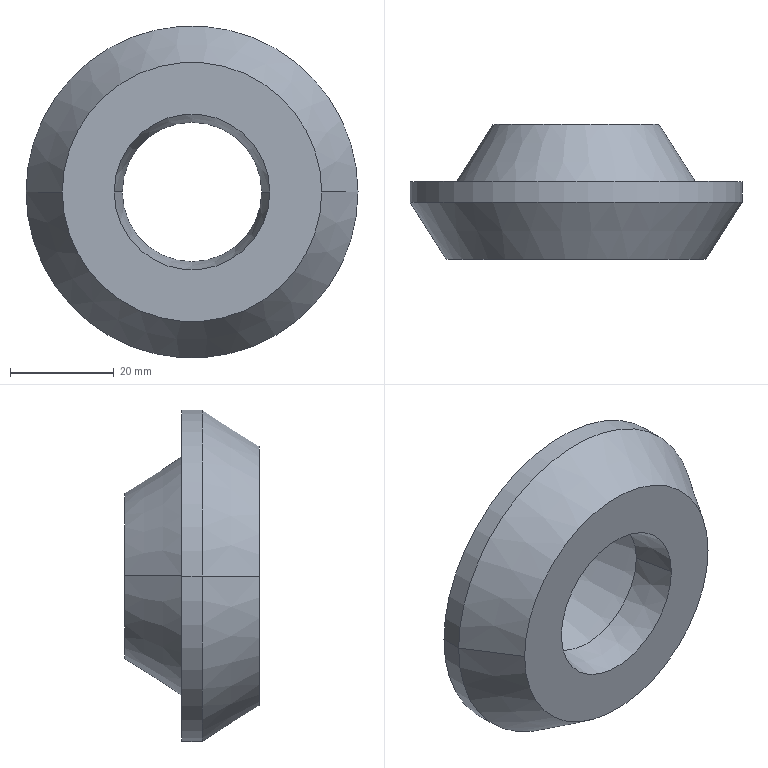Part | SolidWorks | features Revolution 1 | 1 solid | 19 faces | box 64 x 26 x 64 mm | volume 21380 mm3 | cone 12 | plane 5 | cylinder 2 | commonest cylinder face diameters 64 x2
STEP:
#1=CARTESIAN_POINT('',(22.804,4.,0.));
#2=VERTEX_POINT('',#1);
#3=CARTESIAN_POINT('',(-22.804,4.,0.));
#4=VERTEX_POINT('',#3);
#5=CARTESIAN_POINT('',(0.,4.,0.));
#6=DIRECTION('',(0.,1.,0.));
#7=DIRECTION('',(-1.,0.,0.));
#8=AXIS2_PLACEMENT_3D('',#5,#6,#7);
#9=CIRCLE('',#8,22.804);
#10=EDGE_CURVE('',#2,#4,#9,.T.);
#11=ORIENTED_EDGE('',*,*,#10,.F.);
#12=CARTESIAN_POINT('',(27.259,11.,0.));
#13=VERTEX_POINT('',#12);
#14=CARTESIAN_POINT('',(27.259,11.,0.));
#15=DIRECTION('',(0.5369,0.8437,0.));
#16=VECTOR('',#15,1000.);
#17=LINE('',#14,#16);
#18=EDGE_CURVE('',#2,#13,#17,.T.);
#19=ORIENTED_EDGE('',*,*,#18,.T.);
#20=CARTESIAN_POINT('',(-27.259,11.,0.));
#21=VERTEX_POINT('',#20);
#22=CARTESIAN_POINT('',(0.,11.,0.));
#23=DIRECTION('',(0.,1.,0.));
#24=DIRECTION('',(-1.,0.,0.));
#25=AXIS2_PLACEMENT_3D('',#22,#23,#24);
#26=CIRCLE('',#25,27.259);
#27=EDGE_CURVE('',#13,#21,#26,.T.);
#28=ORIENTED_EDGE('',*,*,#27,.T.);
#29=CARTESIAN_POINT('',(-27.259,11.,0.));
#30=DIRECTION('',(-0.5369,0.8437,0.));
#31=VECTOR('',#30,1000.);
#32=LINE('',#29,#31);
#33=EDGE_CURVE('',#4,#21,#32,.T.);
#34=ORIENTED_EDGE('',*,*,#33,.F.);
#35=EDGE_LOOP('',(#11,#19,#28,#34));
#36=FACE_OUTER_BOUND('',#35,.T.);
#37=CARTESIAN_POINT('',(0.,11.,0.));
#38=DIRECTION('',(0.,1.,0.));
#39=DIRECTION('',(-1.,0.,0.));
#40=AXIS2_PLACEMENT_3D('',#37,#38,#39);
#41=CONICAL_SURFACE('',#40,27.259,0.5667);
#42=ADVANCED_FACE('',(#36),#41,.F.);
#43=CARTESIAN_POINT('',(-17.524,8.,0.));
#44=VERTEX_POINT('',#43);
#45=CARTESIAN_POINT('',(17.524,8.,0.));
#46=VERTEX_POINT('',#45);
#47=CARTESIAN_POINT('',(0.,8.,0.));
#48=DIRECTION('',(0.,1.,0.));
#49=DIRECTION('',(-1.,0.,0.));
#50=AXIS2_PLACEMENT_3D('',#47,#48,#49);
#51=CIRCLE('',#50,17.524);
#52=EDGE_CURVE('',#44,#46,#51,.T.);
#53=ORIENTED_EDGE('',*,*,#52,.F.);
#54=CARTESIAN_POINT('',(-18.299,4.,0.));
#55=VERTEX_POINT('',#54);
#56=CARTESIAN_POINT('',(-18.299,4.,0.));
#57=DIRECTION('',(-0.1902,-0.9817,0.));
#58=VECTOR('',#57,1000.);
#59=LINE('',#56,#58);
#60=EDGE_CURVE('',#44,#55,#59,.T.);
#61=ORIENTED_EDGE('',*,*,#60,.T.);
#62=CARTESIAN_POINT('',(18.299,4.,0.));
#63=VERTEX_POINT('',#62);
#64=CARTESIAN_POINT('',(0.,4.,0.));
#65=DIRECTION('',(0.,1.,0.));
#66=DIRECTION('',(-1.,0.,0.));
#67=AXIS2_PLACEMENT_3D('',#64,#65,#66);
#68=CIRCLE('',#67,18.299);
#69=EDGE_CURVE('',#55,#63,#68,.T.);
#70=ORIENTED_EDGE('',*,*,#69,.T.);
#71=CARTESIAN_POINT('',(18.299,4.,0.));
#72=DIRECTION('',(0.1902,-0.9817,0.));
#73=VECTOR('',#72,1000.);
#74=LINE('',#71,#73);
#75=EDGE_CURVE('',#46,#63,#74,.T.);
#76=ORIENTED_EDGE('',*,*,#75,.F.);
#77=EDGE_LOOP('',(#53,#61,#70,#76));
#78=FACE_OUTER_BOUND('',#77,.T.);
#79=CARTESIAN_POINT('',(0.,4.,0.));
#80=DIRECTION('',(0.,-1.,0.));
#81=DIRECTION('',(1.,0.,0.));
#82=AXIS2_PLACEMENT_3D('',#79,#80,#81);
#83=CONICAL_SURFACE('',#82,18.299,0.1914);
#84=ADVANCED_FACE('',(#78),#83,.T.);
#85=CARTESIAN_POINT('',(13.45,8.,0.));
#86=VERTEX_POINT('',#85);
#87=CARTESIAN_POINT('',(-13.45,8.,0.));
#88=VERTEX_POINT('',#87);
#89=CARTESIAN_POINT('',(0.,8.,0.));
#90=DIRECTION('',(0.,1.,0.));
#91=DIRECTION('',(-1.,0.,0.));
#92=AXIS2_PLACEMENT_3D('',#89,#90,#91);
#93=CIRCLE('',#92,13.45);
#94=EDGE_CURVE('',#86,#88,#93,.T.);
#95=ORIENTED_EDGE('',*,*,#94,.T.);
#96=CARTESIAN_POINT('',(-15.,0.,0.));
#97=VERTEX_POINT('',#96);
#98=CARTESIAN_POINT('',(-13.45,8.,0.));
#99=DIRECTION('',(-0.1902,-0.9817,0.));
#100=VECTOR('',#99,1000.);
#101=LINE('',#98,#100);
#102=EDGE_CURVE('',#88,#97,#101,.T.);
#103=ORIENTED_EDGE('',*,*,#102,.T.);
#104=CARTESIAN_POINT('',(15.,0.,0.));
#105=VERTEX_POINT('',#104);
#106=CARTESIAN_POINT('',(0.,0.,0.));
#107=DIRECTION('',(0.,1.,0.));
#108=DIRECTION('',(-1.,0.,0.));
#109=AXIS2_PLACEMENT_3D('',#106,#107,#108);
#110=CIRCLE('',#109,15.);
#111=EDGE_CURVE('',#105,#97,#110,.T.);
#112=ORIENTED_EDGE('',*,*,#111,.F.);
#113=CARTESIAN_POINT('',(13.45,8.,0.));
#114=DIRECTION('',(0.1902,-0.9817,0.));
#115=VECTOR('',#114,1000.);
#116=LINE('',#113,#115);
#117=EDGE_CURVE('',#86,#105,#116,.T.);
#118=ORIENTED_EDGE('',*,*,#117,.F.);
#119=EDGE_LOOP('',(#95,#103,#112,#118));
#120=FACE_OUTER_BOUND('',#119,.T.);
#121=CARTESIAN_POINT('',(0.,8.,0.));
#122=DIRECTION('',(0.,-1.,0.));
#123=DIRECTION('',(1.,0.,0.));
#124=AXIS2_PLACEMENT_3D('',#121,#122,#123);
#125=CONICAL_SURFACE('',#124,13.45,0.1914);
#126=ADVANCED_FACE('',(#120),#125,.F.);
#127=CARTESIAN_POINT('',(-25.,0.,0.));
#128=VERTEX_POINT('',#127);
#129=CARTESIAN_POINT('',(25.,0.,0.));
#130=VERTEX_POINT('',#129);
#131=CARTESIAN_POINT('',(0.,0.,0.));
#132=DIRECTION('',(0.,1.,0.));
#133=DIRECTION('',(-1.,0.,0.));
#134=AXIS2_PLACEMENT_3D('',#131,#132,#133);
#135=CIRCLE('',#134,25.);
#136=EDGE_CURVE('',#128,#130,#135,.T.);
#137=ORIENTED_EDGE('',*,*,#136,.T.);
#138=CARTESIAN_POINT('',(32.,11.,0.));
#139=VERTEX_POINT('',#138);
#140=CARTESIAN_POINT('',(25.,0.,0.));
#141=DIRECTION('',(0.5369,0.8437,0.));
#142=VECTOR('',#141,1000.);
#143=LINE('',#140,#142);
#144=EDGE_CURVE('',#130,#139,#143,.T.);
#145=ORIENTED_EDGE('',*,*,#144,.T.);
#146=CARTESIAN_POINT('',(-32.,11.,0.));
#147=VERTEX_POINT('',#146);
#148=CARTESIAN_POINT('',(0.,11.,0.));
#149=DIRECTION('',(0.,1.,0.));
#150=DIRECTION('',(-1.,0.,0.));
#151=AXIS2_PLACEMENT_3D('',#148,#149,#150);
#152=CIRCLE('',#151,32.);
#153=EDGE_CURVE('',#147,#139,#152,.T.);
#154=ORIENTED_EDGE('',*,*,#153,.F.);
#155=CARTESIAN_POINT('',(-25.,0.,0.));
#156=DIRECTION('',(-0.5369,0.8437,0.));
#157=VECTOR('',#156,1000.);
#158=LINE('',#155,#157);
#159=EDGE_CURVE('',#128,#147,#158,.T.);
#160=ORIENTED_EDGE('',*,*,#159,.F.);
#161=EDGE_LOOP('',(#137,#145,#154,#160));
#162=FACE_OUTER_BOUND('',#161,.T.);
#163=CARTESIAN_POINT('',(0.,0.,0.));
#164=DIRECTION('',(0.,1.,0.));
#165=DIRECTION('',(-1.,0.,0.));
#166=AXIS2_PLACEMENT_3D('',#163,#164,#165);
#167=CONICAL_SURFACE('',#166,25.,0.5667);
#168=ADVANCED_FACE('',(#162),#167,.T.);
#169=ORIENTED_EDGE('',*,*,#153,.T.);
#170=CARTESIAN_POINT('',(32.,15.,0.));
#171=VERTEX_POINT('',#170);
#172=CARTESIAN_POINT('',(32.,12.915,0.));
#173=DIRECTION('',(0.,1.,0.));
#174=VECTOR('',#173,1000.);
#175=LINE('',#172,#174);
#176=EDGE_CURVE('',#139,#171,#175,.T.);
#177=ORIENTED_EDGE('',*,*,#176,.T.);
#178=CARTESIAN_POINT('',(-32.,15.,0.));
#179=VERTEX_POINT('',#178);
#180=CARTESIAN_POINT('',(0.,15.,0.));
#181=DIRECTION('',(0.,1.,0.));
#182=DIRECTION('',(-1.,0.,0.));
#183=AXIS2_PLACEMENT_3D('',#180,#181,#182);
#184=CIRCLE('',#183,32.);
#185=EDGE_CURVE('',#179,#171,#184,.T.);
#186=ORIENTED_EDGE('',*,*,#185,.F.);
#187=CARTESIAN_POINT('',(-32.,12.915,0.));
#188=DIRECTION('',(0.,1.,0.));
#189=VECTOR('',#188,1000.);
#190=LINE('',#187,#189);
#191=EDGE_CURVE('',#147,#179,#190,.T.);
#192=ORIENTED_EDGE('',*,*,#191,.F.);
#193=EDGE_LOOP('',(#169,#177,#186,#192));
#194=FACE_OUTER_BOUND('',#193,.T.);
#195=CARTESIAN_POINT('',(0.,12.915,0.));
#196=DIRECTION('',(0.,1.,0.));
#197=DIRECTION('',(-1.,0.,0.));
#198=AXIS2_PLACEMENT_3D('',#195,#196,#197);
#199=CYLINDRICAL_SURFACE('',#198,32.);
#200=ADVANCED_FACE('',(#194),#199,.T.);
#201=CARTESIAN_POINT('',(-16.,26.,0.));
#202=VERTEX_POINT('',#201);
#203=CARTESIAN_POINT('',(16.,26.,0.));
#204=VERTEX_POINT('',#203);
#205=CARTESIAN_POINT('',(0.,26.,0.));
#206=DIRECTION('',(0.,1.,0.));
#207=DIRECTION('',(-1.,0.,0.));
#208=AXIS2_PLACEMENT_3D('',#205,#206,#207);
#209=CIRCLE('',#208,16.);
#210=EDGE_CURVE('',#202,#204,#209,.T.);
#211=ORIENTED_EDGE('',*,*,#210,.F.);
#212=CARTESIAN_POINT('',(-23.,15.,0.));
#213=VERTEX_POINT('',#212);
#214=CARTESIAN_POINT('',(-23.,15.,0.));
#215=DIRECTION('',(-0.5369,-0.8437,0.));
#216=VECTOR('',#215,1000.);
#217=LINE('',#214,#216);
#218=EDGE_CURVE('',#202,#213,#217,.T.);
#219=ORIENTED_EDGE('',*,*,#218,.T.);
#220=CARTESIAN_POINT('',(23.,15.,0.));
#221=VERTEX_POINT('',#220);
#222=CARTESIAN_POINT('',(0.,15.,0.));
#223=DIRECTION('',(0.,1.,0.));
#224=DIRECTION('',(-1.,0.,0.));
#225=AXIS2_PLACEMENT_3D('',#222,#223,#224);
#226=CIRCLE('',#225,23.);
#227=EDGE_CURVE('',#213,#221,#226,.T.);
#228=ORIENTED_EDGE('',*,*,#227,.T.);
#229=CARTESIAN_POINT('',(23.,15.,0.));
#230=DIRECTION('',(0.5369,-0.8437,0.));
#231=VECTOR('',#230,1000.);
#232=LINE('',#229,#231);
#233=EDGE_CURVE('',#204,#221,#232,.T.);
#234=ORIENTED_EDGE('',*,*,#233,.F.);
#235=EDGE_LOOP('',(#211,#219,#228,#234));
#236=FACE_OUTER_BOUND('',#235,.T.);
#237=CARTESIAN_POINT('',(0.,15.,0.));
#238=DIRECTION('',(0.,-1.,0.));
#239=DIRECTION('',(1.,0.,0.));
#240=AXIS2_PLACEMENT_3D('',#237,#238,#239);
#241=CONICAL_SURFACE('',#240,23.,0.5667);
#242=ADVANCED_FACE('',(#236),#241,.T.);
#243=CARTESIAN_POINT('',(0.,26.,0.));
#244=DIRECTION('',(0.,1.,0.));
#245=DIRECTION('',(-1.,0.,0.));
#246=AXIS2_PLACEMENT_3D('',#243,#244,#245);
#247=CIRCLE('',#246,16.);
#248=EDGE_CURVE('',#204,#202,#247,.T.);
#249=ORIENTED_EDGE('',*,*,#248,.T.);
#250=CARTESIAN_POINT('',(-22.995,11.,0.));
#251=VERTEX_POINT('',#250);
#252=CARTESIAN_POINT('',(-16.,26.,0.));
#253=DIRECTION('',(-0.4226,-0.9063,0.));
#254=VECTOR('',#253,1000.);
#255=LINE('',#252,#254);
#256=EDGE_CURVE('',#202,#251,#255,.T.);
#257=ORIENTED_EDGE('',*,*,#256,.T.);
#258=CARTESIAN_POINT('',(22.995,11.,0.));
#259=VERTEX_POINT('',#258);
#260=CARTESIAN_POINT('',(0.,11.,0.));
#261=DIRECTION('',(0.,1.,0.));
#262=DIRECTION('',(-1.,0.,0.));
#263=AXIS2_PLACEMENT_3D('',#260,#261,#262);
#264=CIRCLE('',#263,22.995);
#265=EDGE_CURVE('',#259,#251,#264,.T.);
#266=ORIENTED_EDGE('',*,*,#265,.F.);
#267=CARTESIAN_POINT('',(16.,26.,0.));
#268=DIRECTION('',(0.4226,-0.9063,0.));
#269=VECTOR('',#268,1000.);
#270=LINE('',#267,#269);
#271=EDGE_CURVE('',#204,#259,#270,.T.);
#272=ORIENTED_EDGE('',*,*,#271,.F.);
#273=EDGE_LOOP('',(#249,#257,#266,#272));
#274=FACE_OUTER_BOUND('',#273,.T.);
#275=CARTESIAN_POINT('',(0.,26.,0.));
#276=DIRECTION('',(0.,-1.,0.));
#277=DIRECTION('',(1.,0.,0.));
#278=AXIS2_PLACEMENT_3D('',#275,#276,#277);
#279=CONICAL_SURFACE('',#278,16.,0.4363);
#280=ADVANCED_FACE('',(#274),#279,.F.);
#281=ORIENTED_EDGE('',*,*,#256,.F.);
#282=ORIENTED_EDGE('',*,*,#210,.T.);
#283=ORIENTED_EDGE('',*,*,#271,.T.);
#284=CARTESIAN_POINT('',(0.,11.,0.));
#285=DIRECTION('',(0.,1.,0.));
#286=DIRECTION('',(-1.,0.,0.));
#287=AXIS2_PLACEMENT_3D('',#284,#285,#286);
#288=CIRCLE('',#287,22.995);
#289=EDGE_CURVE('',#251,#259,#288,.T.);
#290=ORIENTED_EDGE('',*,*,#289,.F.);
#291=EDGE_LOOP('',(#281,#282,#283,#290));
#292=FACE_OUTER_BOUND('',#291,.T.);
#293=CARTESIAN_POINT('',(0.,26.,0.));
#294=DIRECTION('',(0.,-1.,0.));
#295=DIRECTION('',(1.,0.,0.));
#296=AXIS2_PLACEMENT_3D('',#293,#294,#295);
#297=CONICAL_SURFACE('',#296,16.,0.4363);
#298=ADVANCED_FACE('',(#292),#297,.F.);
#299=ORIENTED_EDGE('',*,*,#218,.F.);
#300=ORIENTED_EDGE('',*,*,#248,.F.);
#301=ORIENTED_EDGE('',*,*,#233,.T.);
#302=CARTESIAN_POINT('',(0.,15.,0.));
#303=DIRECTION('',(0.,1.,0.));
#304=DIRECTION('',(-1.,0.,0.));
#305=AXIS2_PLACEMENT_3D('',#302,#303,#304);
#306=CIRCLE('',#305,23.);
#307=EDGE_CURVE('',#221,#213,#306,.T.);
#308=ORIENTED_EDGE('',*,*,#307,.T.);
#309=EDGE_LOOP('',(#299,#300,#301,#308));
#310=FACE_OUTER_BOUND('',#309,.T.);
#311=CARTESIAN_POINT('',(0.,15.,0.));
#312=DIRECTION('',(0.,-1.,0.));
#313=DIRECTION('',(1.,0.,0.));
#314=AXIS2_PLACEMENT_3D('',#311,#312,#313);
#315=CONICAL_SURFACE('',#314,23.,0.5667);
#316=ADVANCED_FACE('',(#310),#315,.T.);
#317=ORIENTED_EDGE('',*,*,#307,.F.);
#318=ORIENTED_EDGE('',*,*,#227,.F.);
#319=EDGE_LOOP('',(#317,#318));
#320=FACE_BOUND('',#319,.T.);
#321=ORIENTED_EDGE('',*,*,#185,.T.);
#322=CARTESIAN_POINT('',(0.,15.,0.));
#323=DIRECTION('',(0.,1.,0.));
#324=DIRECTION('',(-1.,0.,0.));
#325=AXIS2_PLACEMENT_3D('',#322,#323,#324);
#326=CIRCLE('',#325,32.);
#327=EDGE_CURVE('',#171,#179,#326,.T.);
#328=ORIENTED_EDGE('',*,*,#327,.T.);
#329=EDGE_LOOP('',(#321,#328));
#330=FACE_OUTER_BOUND('',#329,.T.);
#331=CARTESIAN_POINT('',(23.,15.,0.));
#332=DIRECTION('',(0.,-1.,0.));
#333=DIRECTION('',(1.,0.,0.));
#334=AXIS2_PLACEMENT_3D('',#331,#332,#333);
#335=PLANE('',#334);
#336=ADVANCED_FACE('',(#320,#330),#335,.F.);
#337=ORIENTED_EDGE('',*,*,#176,.F.);
#338=CARTESIAN_POINT('',(0.,11.,0.));
#339=DIRECTION('',(0.,1.,0.));
#340=DIRECTION('',(-1.,0.,0.));
#341=AXIS2_PLACEMENT_3D('',#338,#339,#340);
#342=CIRCLE('',#341,32.);
#343=EDGE_CURVE('',#139,#147,#342,.T.);
#344=ORIENTED_EDGE('',*,*,#343,.T.);
#345=ORIENTED_EDGE('',*,*,#191,.T.);
#346=ORIENTED_EDGE('',*,*,#327,.F.);
#347=EDGE_LOOP('',(#337,#344,#345,#346));
#348=FACE_OUTER_BOUND('',#347,.T.);
#349=CARTESIAN_POINT('',(0.,12.915,0.));
#350=DIRECTION('',(0.,1.,0.));
#351=DIRECTION('',(-1.,0.,0.));
#352=AXIS2_PLACEMENT_3D('',#349,#350,#351);
#353=CYLINDRICAL_SURFACE('',#352,32.);
#354=ADVANCED_FACE('',(#348),#353,.T.);
#355=ORIENTED_EDGE('',*,*,#144,.F.);
#356=CARTESIAN_POINT('',(0.,0.,0.));
#357=DIRECTION('',(0.,1.,0.));
#358=DIRECTION('',(-1.,0.,0.));
#359=AXIS2_PLACEMENT_3D('',#356,#357,#358);
#360=CIRCLE('',#359,25.);
#361=EDGE_CURVE('',#130,#128,#360,.T.);
#362=ORIENTED_EDGE('',*,*,#361,.T.);
#363=ORIENTED_EDGE('',*,*,#159,.T.);
#364=ORIENTED_EDGE('',*,*,#343,.F.);
#365=EDGE_LOOP('',(#355,#362,#363,#364));
#366=FACE_OUTER_BOUND('',#365,.T.);
#367=CARTESIAN_POINT('',(0.,0.,0.));
#368=DIRECTION('',(0.,1.,0.));
#369=DIRECTION('',(-1.,0.,0.));
#370=AXIS2_PLACEMENT_3D('',#367,#368,#369);
#371=CONICAL_SURFACE('',#370,25.,0.5667);
#372=ADVANCED_FACE('',(#366),#371,.T.);
#373=ORIENTED_EDGE('',*,*,#136,.F.);
#374=ORIENTED_EDGE('',*,*,#361,.F.);
#375=EDGE_LOOP('',(#373,#374));
#376=FACE_OUTER_BOUND('',#375,.T.);
#377=ORIENTED_EDGE('',*,*,#111,.T.);
#378=CARTESIAN_POINT('',(0.,0.,0.));
#379=DIRECTION('',(0.,1.,0.));
#380=DIRECTION('',(-1.,0.,0.));
#381=AXIS2_PLACEMENT_3D('',#378,#379,#380);
#382=CIRCLE('',#381,15.);
#383=EDGE_CURVE('',#97,#105,#382,.T.);
#384=ORIENTED_EDGE('',*,*,#383,.T.);
#385=EDGE_LOOP('',(#377,#384));
#386=FACE_BOUND('',#385,.T.);
#387=CARTESIAN_POINT('',(25.,0.,0.));
#388=DIRECTION('',(0.,1.,0.));
#389=DIRECTION('',(-1.,0.,0.));
#390=AXIS2_PLACEMENT_3D('',#387,#388,#389);
#391=PLANE('',#390);
#392=ADVANCED_FACE('',(#376,#386),#391,.F.);
#393=ORIENTED_EDGE('',*,*,#102,.F.);
#394=CARTESIAN_POINT('',(0.,8.,0.));
#395=DIRECTION('',(0.,1.,0.));
#396=DIRECTION('',(-1.,0.,0.));
#397=AXIS2_PLACEMENT_3D('',#394,#395,#396);
#398=CIRCLE('',#397,13.45);
#399=EDGE_CURVE('',#88,#86,#398,.T.);
#400=ORIENTED_EDGE('',*,*,#399,.T.);
#401=ORIENTED_EDGE('',*,*,#117,.T.);
#402=ORIENTED_EDGE('',*,*,#383,.F.);
#403=EDGE_LOOP('',(#393,#400,#401,#402));
#404=FACE_OUTER_BOUND('',#403,.T.);
#405=CARTESIAN_POINT('',(0.,8.,0.));
#406=DIRECTION('',(0.,-1.,0.));
#407=DIRECTION('',(1.,0.,0.));
#408=AXIS2_PLACEMENT_3D('',#405,#406,#407);
#409=CONICAL_SURFACE('',#408,13.45,0.1914);
#410=ADVANCED_FACE('',(#404),#409,.F.);
#411=ORIENTED_EDGE('',*,*,#94,.F.);
#412=ORIENTED_EDGE('',*,*,#399,.F.);
#413=EDGE_LOOP('',(#411,#412));
#414=FACE_BOUND('',#413,.T.);
#415=CARTESIAN_POINT('',(0.,8.,0.));
#416=DIRECTION('',(0.,1.,0.));
#417=DIRECTION('',(-1.,0.,0.));
#418=AXIS2_PLACEMENT_3D('',#415,#416,#417);
#419=CIRCLE('',#418,17.524);
#420=EDGE_CURVE('',#46,#44,#419,.T.);
#421=ORIENTED_EDGE('',*,*,#420,.T.);
#422=ORIENTED_EDGE('',*,*,#52,.T.);
#423=EDGE_LOOP('',(#421,#422));
#424=FACE_OUTER_BOUND('',#423,.T.);
#425=CARTESIAN_POINT('',(13.45,8.,0.));
#426=DIRECTION('',(0.,-1.,0.));
#427=DIRECTION('',(1.,0.,0.));
#428=AXIS2_PLACEMENT_3D('',#425,#426,#427);
#429=PLANE('',#428);
#430=ADVANCED_FACE('',(#414,#424),#429,.F.);
#431=ORIENTED_EDGE('',*,*,#60,.F.);
#432=ORIENTED_EDGE('',*,*,#420,.F.);
#433=ORIENTED_EDGE('',*,*,#75,.T.);
#434=CARTESIAN_POINT('',(0.,4.,0.));
#435=DIRECTION('',(0.,1.,0.));
#436=DIRECTION('',(-1.,0.,0.));
#437=AXIS2_PLACEMENT_3D('',#434,#435,#436);
#438=CIRCLE('',#437,18.299);
#439=EDGE_CURVE('',#63,#55,#438,.T.);
#440=ORIENTED_EDGE('',*,*,#439,.T.);
#441=EDGE_LOOP('',(#431,#432,#433,#440));
#442=FACE_OUTER_BOUND('',#441,.T.);
#443=CARTESIAN_POINT('',(0.,4.,0.));
#444=DIRECTION('',(0.,-1.,0.));
#445=DIRECTION('',(1.,0.,0.));
#446=AXIS2_PLACEMENT_3D('',#443,#444,#445);
#447=CONICAL_SURFACE('',#446,18.299,0.1914);
#448=ADVANCED_FACE('',(#442),#447,.T.);
#449=ORIENTED_EDGE('',*,*,#439,.F.);
#450=ORIENTED_EDGE('',*,*,#69,.F.);
#451=EDGE_LOOP('',(#449,#450));
#452=FACE_BOUND('',#451,.T.);
#453=CARTESIAN_POINT('',(0.,4.,0.));
#454=DIRECTION('',(0.,1.,0.));
#455=DIRECTION('',(-1.,0.,0.));
#456=AXIS2_PLACEMENT_3D('',#453,#454,#455);
#457=CIRCLE('',#456,22.804);
#458=EDGE_CURVE('',#4,#2,#457,.T.);
#459=ORIENTED_EDGE('',*,*,#458,.T.);
#460=ORIENTED_EDGE('',*,*,#10,.T.);
#461=EDGE_LOOP('',(#459,#460));
#462=FACE_OUTER_BOUND('',#461,.T.);
#463=CARTESIAN_POINT('',(18.299,4.,0.));
#464=DIRECTION('',(0.,-1.,0.));
#465=DIRECTION('',(1.,0.,0.));
#466=AXIS2_PLACEMENT_3D('',#463,#464,#465);
#467=PLANE('',#466);
#468=ADVANCED_FACE('',(#452,#462),#467,.F.);
#469=ORIENTED_EDGE('',*,*,#18,.F.);
#470=ORIENTED_EDGE('',*,*,#458,.F.);
#471=ORIENTED_EDGE('',*,*,#33,.T.);
#472=CARTESIAN_POINT('',(0.,11.,0.));
#473=DIRECTION('',(0.,1.,0.));
#474=DIRECTION('',(-1.,0.,0.));
#475=AXIS2_PLACEMENT_3D('',#472,#473,#474);
#476=CIRCLE('',#475,27.259);
#477=EDGE_CURVE('',#21,#13,#476,.T.);
#478=ORIENTED_EDGE('',*,*,#477,.T.);
#479=EDGE_LOOP('',(#469,#470,#471,#478));
#480=FACE_OUTER_BOUND('',#479,.T.);
#481=CARTESIAN_POINT('',(0.,11.,0.));
#482=DIRECTION('',(0.,1.,0.));
#483=DIRECTION('',(-1.,0.,0.));
#484=AXIS2_PLACEMENT_3D('',#481,#482,#483);
#485=CONICAL_SURFACE('',#484,27.259,0.5667);
#486=ADVANCED_FACE('',(#480),#485,.F.);
#487=ORIENTED_EDGE('',*,*,#477,.F.);
#488=ORIENTED_EDGE('',*,*,#27,.F.);
#489=EDGE_LOOP('',(#487,#488));
#490=FACE_OUTER_BOUND('',#489,.T.);
#491=ORIENTED_EDGE('',*,*,#265,.T.);
#492=ORIENTED_EDGE('',*,*,#289,.T.);
#493=EDGE_LOOP('',(#491,#492));
#494=FACE_BOUND('',#493,.T.);
#495=CARTESIAN_POINT('',(27.259,11.,0.));
#496=DIRECTION('',(0.,1.,0.));
#497=DIRECTION('',(-1.,0.,0.));
#498=AXIS2_PLACEMENT_3D('',#495,#496,#497);
#499=PLANE('',#498);
#500=ADVANCED_FACE('',(#490,#494),#499,.F.);
#501=CLOSED_SHELL('',(#42,#84,#126,#168,#200,#242,#280,#298,#316,#336,#354,#372,#392,#410,#430,#448,#468,#486,#500));
#502=MANIFOLD_SOLID_BREP('',#501);
#503=CARTESIAN_POINT('',(0.,0.,0.));
#504=DIRECTION('',(0.,0.,1.));
#505=DIRECTION('',(1.,0.,0.));
#506=AXIS2_PLACEMENT_3D('',#503,#504,#505);
#507=(LENGTH_UNIT()NAMED_UNIT(*)SI_UNIT(.MILLI.,.METRE.));
#508=UNCERTAINTY_MEASURE_WITH_UNIT(LENGTH_MEASURE(0.00001),#507,'','');
#509=(NAMED_UNIT(*)PLANE_ANGLE_UNIT()SI_UNIT($,.RADIAN.));
#510=(NAMED_UNIT(*)SI_UNIT($,.STERADIAN.)SOLID_ANGLE_UNIT());
#511=(GEOMETRIC_REPRESENTATION_CONTEXT(3)GLOBAL_UNCERTAINTY_ASSIGNED_CONTEXT((#508))GLOBAL_UNIT_ASSIGNED_CONTEXT((#507,#509,#510))REPRESENTATION_CONTEXT('',''));
#512=ADVANCED_BREP_SHAPE_REPRESENTATION('',(#502,#506),#511);